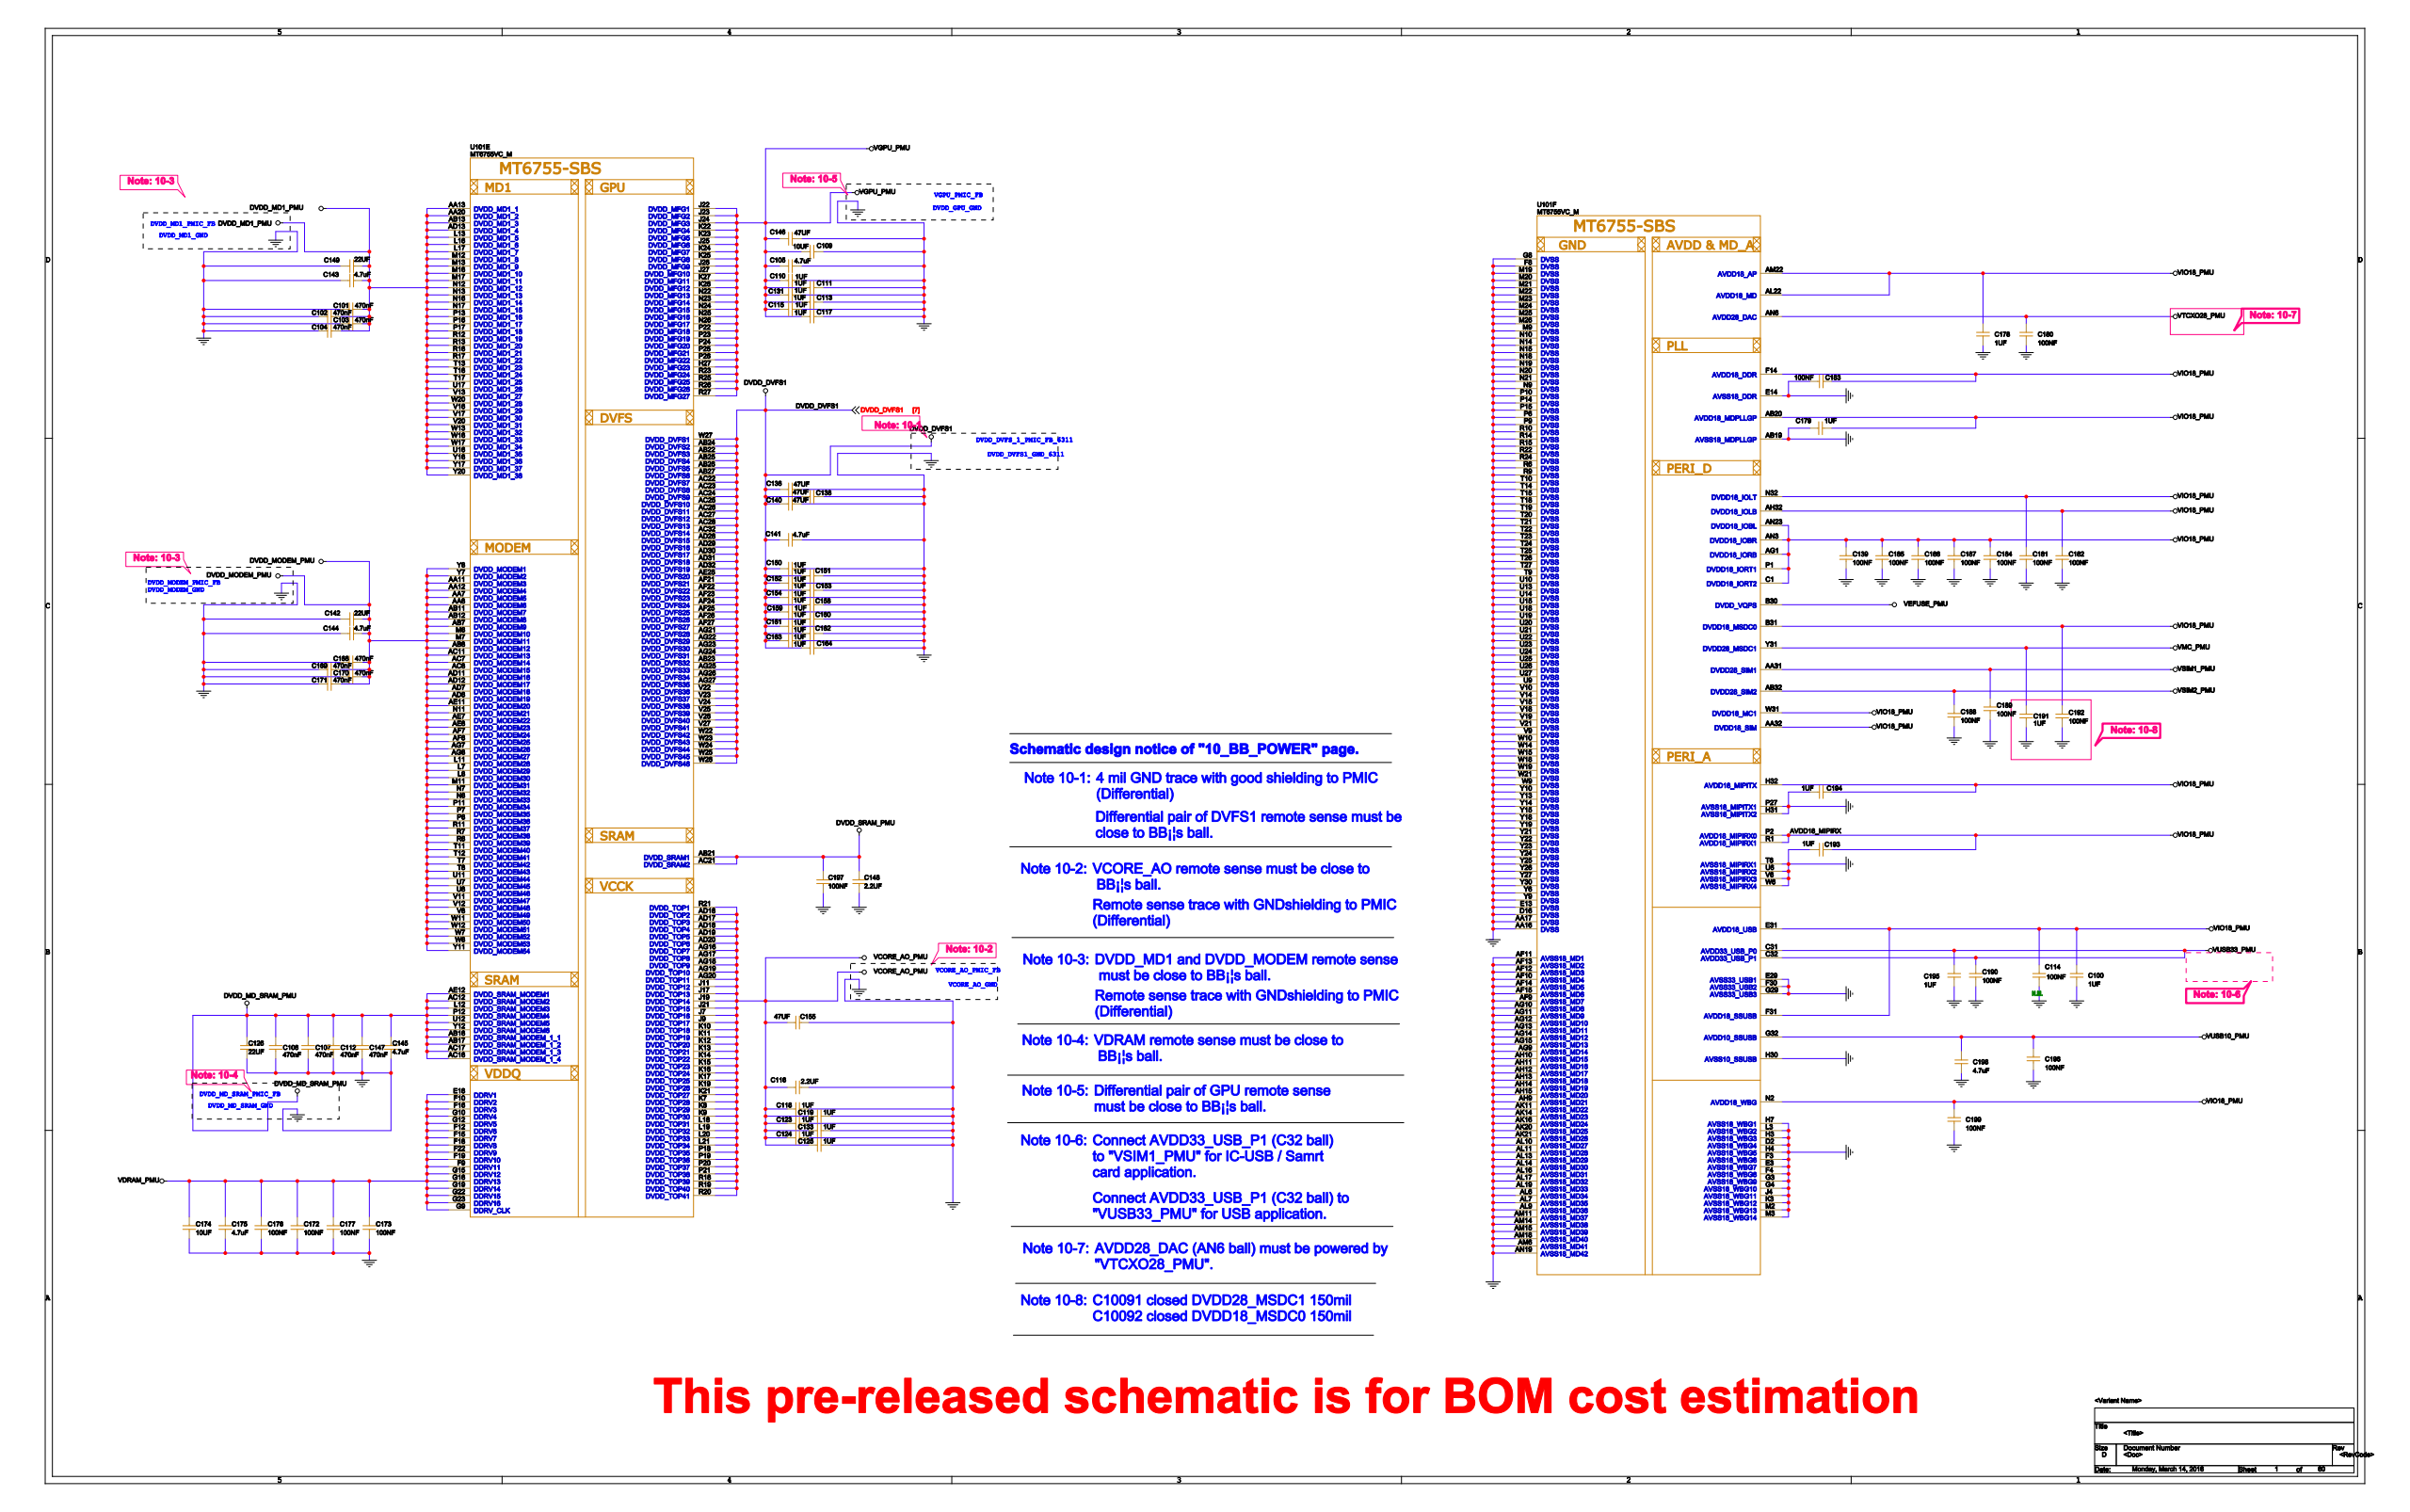Circuit board | Cadence Allegro | 1088 parts | 793 nets | one sheet of the schematic
Parts on this sheet (reference | value | footprint):
C100 | 1UF | C0201
C101 | 470nF | C0201
C102 | 470nF | C0201
C103 | 470nF | C0201
C104 | 470nF | C0201
C105 | 4.7uF | 0402-BIG
C106 | 470nF | C0201
C107 | 470nF | C0201
C109 | 10UF | 0603-BIG
C110 | 1UF | C0201
C111 | 1UF | C0201
C112 | 470nF | C0201
C113 | 1UF | C0201
C114
C115 | 1UF | C0201
C116 | 2.2UF | 0402-BIG
C117 | 1UF | C0201
C118 | 1UF | C0201
C119 | 1UF | C0201
C123 | 1UF | C0201
C124 | 1UF | C0201
C125 | 1UF | C0201
C126 | 22UF | 0603-BIG
C131 | 1UF | C0201
C133 | 1UF | C0201
C136 | 47UF | 0603-BIG
C138 | 47UF | 0603-BIG
C139 | 100NF | C0201
C140 | 47UF | 0603-BIG
C141 | 4.7uF | 0402-BIG
C142 | 22UF | 0603-BIG
C143 | 4.7uF | 0402-BIG
C144 | 4.7uF | 0402-BIG
C145 | 4.7uF | 0402-BIG
C146 | 47UF | 0603-BIG
C147 | 470nF | C0201
C148 | 2.2UF | 0402-BIG
C149 | 22UF | 0603-BIG
C150 | 1UF | C0201
C151 | 1UF | C0201
C152 | 1UF | C0201
C153 | 1UF | C0201
C154 | 1UF | C0201
C155 | 47UF | 0603-BIG
C158 | 1UF | C0201
C159 | 1UF | C0201
C160 | 1UF | C0201
C161 | 1UF | C0201
C162 | 1UF | C0201
C163 | 1UF | C0201
C164 | 1UF | C0201
C168 | 470nF | C0201
C169 | 470nF | C0201
C170 | 470nF | C0201
C171 | 470nF | C0201
C172 | 100NF | C0201
C173 | 100NF | C0201
C174 | 10UF | 0603-BIG
C175 | 4.7uF | 0402-BIG
C176 | 100NF | C0201
C177 | 100NF | C0201
C178 | 1UF | C0201
C179 | 1UF | C0201
C180 | 100NF | C0201
C181 | 100NF | C0201
C182 | 100NF | C0201
C183 | 100NF | C0201
C184 | 100NF | C0201
C185 | 100NF | C0201
C186 | 100NF | C0201
C187 | 100NF | C0201
C188 | 100NF | C0201
C189 | 100NF | C0201
C190 | 100NF | C0201
C191 | 1UF | C0201
C192 | 100NF | C0201
C193 | 1UF | C0201
C194 | 1UF | C0201
C195 | 1UF | C0201
C196 | 100NF | C0201
C197 | 100NF | C0201
C198 | 4.7uF | 0402-BIG
C199 | 100NF | C0201
U101 | MT6755VC_M | MT6755
Nets of these parts (net: part-pin ...):
GND: C100-2 C101-1 C102-1 C103-1 C104-1 C105-2 C106-2 C107-2 C109-2 C110-2 C111-2 C112-2 C113-2 C114-2 C115-2 C116-2 C117-2 C118-2 C119-2 C123-2 C124-2 C125-2 C126-2 C131-2 C133-2 C136-2 C138-2 C139-2 C140-2 C141-2 C142-2 C143-2 C144-2 C145-2 C146-2 C147-2 C148-2 C149-2 C150-2 C151-2 C152-2 C153-2 C154-2 C155-2 C158-2 C159-2 C160-2 C161-2 C162-2 C163-2 C164-2 C168-1 C169-1 C170-1 C171-1 C172-2 C173-2 C174-2 C175-2 C176-2 C177-2 C178-2 C179-1 C180-2 C181-2 C182-2 C183-2 C184-2 C185-2 C186-2 C187-2 C188-2 C189-2 C190-2 C191-2 C192-2 C193-2 C194-2 C195-2 C196-2 C197-2 C198-2 C199-2 U101-AA16 U101-AA17 U101-AB19 U101-AF9 U101-AF10 U101-AF11 U101-AF12 U101-AF13 U101-AF14 U101-AF15 U101-AG9 U101-AG10 U101-AG11 U101-AG12 U101-AG13 U101-AG14 U101-AG15 U101-AH9 U101-AH10 U101-AH11 U101-AH12 U101-AH13 U101-AH14 U101-AH15 U101-AK11 U101-AK14 U101-AK16 U101-AK20 U101-AK21 U101-AL6 U101-AL7 U101-AL9 U101-AL10 U101-AL11 U101-AL13 U101-AL14 U101-AL16 U101-AL17 U101-AL19 U101-AM6 U101-AM11 U101-AM14 U101-AM15 U101-AM18 U101-AN19 U101-D2 U101-D16 U101-E3 U101-E13 U101-E14 U101-E29 U101-F3 U101-F4 U101-F8 U101-F30 U101-G3 U101-G4 U101-G8 U101-G29 U101-H3 U101-H4 U101-H7 U101-H30 U101-H31 U101-J4 U101-K3 U101-L3 U101-M2 U101-M3 U101-M9 U101-M19 U101-M20 U101-M21 U101-M22 U101-M23 U101-M24 U101-M25 U101-M26 U101-N9 U101-N10 U101-N14 U101-N15 U101-N18 U101-N19 U101-N20 U101-N21 U101-P6 U101-P9 U101-P10 U101-P14 U101-P15 U101-P27 U101-R6 U101-R9 U101-R10 U101-R14 U101-R15 U101-R22 U101-R24 U101-T6 U101-T9 U101-T10 U101-T14 U101-T15 U101-T18 U101-T19 U101-T20 U101-T21 U101-T22 U101-T23 U101-T24 U101-T25 U101-T26 U101-T27 U101-U6 U101-U9 U101-U10 U101-U13 U101-U14 U101-U15 U101-U18 U101-U19 U101-U20 U101-U21 U101-U22 U101-U23 U101-U24 U101-U25 U101-U26 U101-U27 U101-V6 U101-V9 U101-V10 U101-V14 U101-V15 U101-V18 U101-V19 U101-V21 U101-W6 U101-W9 U101-W10 U101-W14 U101-W15 U101-W18 U101-W19 U101-W21 U101-Y6 U101-Y9 U101-Y10 U101-Y13 U101-Y14 U101-Y15 U101-Y18 U101-Y19 U101-Y21 U101-Y22 U101-Y23 U101-Y24 U101-Y25 U101-Y26 U101-Y27 U101-Y30
VDRAM_PMU: C172-1 C173-1 C174-1 C175-1 C176-1 C177-1 U101-E18 U101-F9 U101-F10 U101-F12 U101-F15 U101-F16 U101-F18 U101-F19 U101-F22 U101-G9 U101-G10 U101-G12 U101-G15 U101-G16 U101-G19 U101-G22 U101-G23
DVDD_DVFS1: C136-1 C138-1 C140-1 C141-1 C150-1 C151-1 C152-1 C153-1 C154-1 C158-1 C159-1 C160-1 C161-1 C162-1 C163-1 C164-1 U101-AB22 U101-AB23 U101-AB24 U101-AB25 U101-AB26 U101-AB27 U101-AC22 U101-AC23 U101-AC24 U101-AC25 U101-AC26 U101-AC27 U101-AC28 U101-AC32 U101-AD28 U101-AD29 U101-AD30 U101-AD31 U101-AD32 U101-AE28 U101-AF21 U101-AF22 U101-AF23 U101-AF24 U101-AF25 U101-AF26 U101-AF27 U101-AG21 U101-AG22 U101-AG23 U101-AG24 U101-AG25 U101-AG26 U101-AG27 U101-V22 U101-V23 U101-V24 U101-V25 U101-V26 U101-V27 U101-W22 U101-W23 U101-W24 U101-W25 U101-W26 U101-W27
DVDD_MD1_PMU: C101-2 C102-2 C103-2 C104-2 C143-1 C149-1 U101-AA13 U101-AA20 U101-AB13 U101-AD13 U101-L13 U101-L16 U101-L17 U101-M12 U101-M13 U101-M16 U101-M17 U101-N12 U101-N13 U101-N16 U101-N17 U101-P13 U101-P16 U101-P17 U101-R12 U101-R13 U101-R16 U101-R17 U101-T13 U101-T16 U101-T17 U101-U16 U101-U17 U101-V13 U101-V16 U101-V17 U101-V20 U101-W13 U101-W16 U101-W17 U101-W20 U101-Y16 U101-Y17 U101-Y20
VGPU_PMU: C105-1 C109-1 C110-1 C111-1 C113-1 C115-1 C117-1 C131-1 C146-1 U101-H27 U101-J22 U101-J23 U101-J24 U101-J25 U101-J26 U101-J27 U101-K22 U101-K23 U101-K24 U101-K25 U101-K26 U101-K27 U101-N22 U101-N23 U101-N24 U101-N25 U101-N26 U101-P22 U101-P23 U101-P24 U101-P25 U101-P26 U101-R23 U101-R25 U101-R26 U101-R27
DVDD_MODEM_PMU: C142-1 C144-1 C168-2 C169-2 C170-2 C171-2 U101-AA7 U101-AA8 U101-AA11 U101-AA12 U101-AB7 U101-AB8 U101-AB11 U101-AB12 U101-AC7 U101-AC8 U101-AC11 U101-AD7 U101-AD8 U101-AD11 U101-AD12 U101-AE7 U101-AE8 U101-AE11 U101-AF7 U101-AF8 U101-AG7 U101-AG8 U101-L7 U101-L8 U101-L11 U101-M7 U101-M8 U101-M11 U101-N7 U101-N8 U101-N11 U101-P7 U101-P8 U101-P11 U101-R7 U101-R8 U101-R11 U101-T7 U101-T8 U101-T11 U101-T12 U101-U7 U101-U8 U101-U11 U101-V8 U101-V11 U101-V12 U101-W7 U101-W8 U101-W11 U101-W12 U101-Y7 U101-Y8 U101-Y11
DVDD_SRAM_PMU: C148-1 C197-1 U101-AB21 U101-AC21
DVDD_MD_SRAM_PMU: C106-1 C107-1 C112-1 C126-1 C145-1 C147-1 U101-AB16 U101-AB17 U101-AC12 U101-AC16 U101-AC17 U101-AE12 U101-L12 U101-P12 U101-U12 U101-Y12
VCORE_AO_PMU: C116-1 C118-1 C119-1 C123-1 C124-1 C125-1 C133-1 C155-1 U101-AD16 U101-AD17 U101-AD18 U101-AD19 U101-AD20 U101-AG16 U101-AG17 U101-AG18 U101-AG19 U101-AG20 U101-J7 U101-J9 U101-J11 U101-J17 U101-J19 U101-J21 U101-K7 U101-K8 U101-K9 U101-K10 U101-K11 U101-K12 U101-K13 U101-K14 U101-K15 U101-K16 U101-K17 U101-K19 U101-K21 U101-L18 U101-L19 U101-L20 U101-L21 U101-P18 U101-P19 U101-P20 U101-P21 U101-R18 U101-R19 U101-R20 U101-R21
VUSB10_PMU: C196-1 C198-1 U101-G32
VIO18_PMU: C100-1 C114-1 C139-1 C178-1 C179-2 C181-1 C182-1 C183-1 C184-1 C185-1 C186-1 C187-1 C192-1 C193-1 C194-1 C199-1 U101-AA32 U101-AB20 U101-AG1 U101-AH32 U101-AL22 U101-AM22 U101-AN3 U101-AN23 U101-B31 U101-C1 U101-E31 U101-F14 U101-F31 U101-H32 U101-N2 U101-N32 U101-P1 U101-P2 U101-R1 U101-W31
VTCXO28_PMU: C180-1 U101-AN6
VUSB33_PMU: C190-1 C195-1 U101-C31 U101-C32
VMC_PMU: C191-1 U101-Y31
VSIM1_PMU: C189-1 U101-AA31
VSIM2_PMU: C188-1 U101-AB32
VEFUSE_PMU: U101-B30